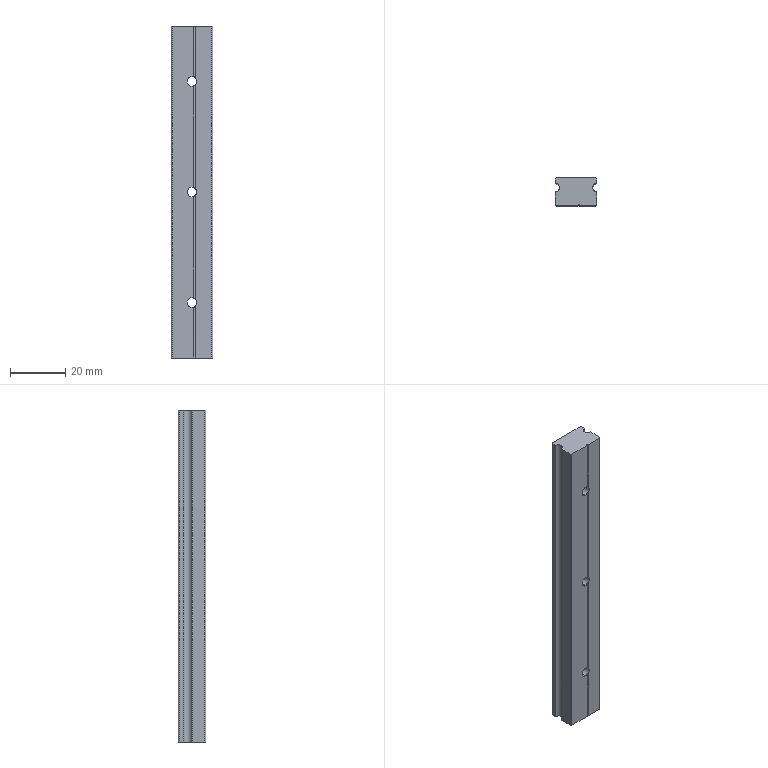Part | STEP file | MGN15H-120-01 | 1 solid | 35 faces | box 15 x 10 x 120 mm | volume 16613 mm3 | cylinder 19 | plane 16 | commonest cylinder face diameters 3.5 x6 6 x6 0.6 x4 3 x3